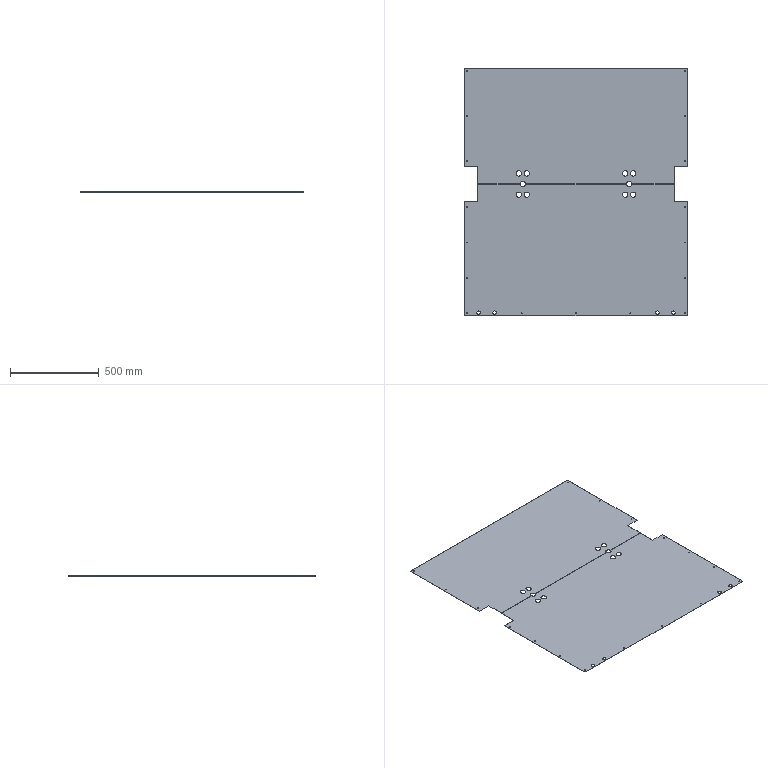Part | SolidWorks | features ICE 4, FlatPattern 2, Cut 1, Fillet 1, MirrorPattern 1, SMBaseFlange 1, SheetMetal 1 | 2 solids | 88 faces | box 1260 x 1400 x 1 mm | volume 1723179 mm3 | cylinder 64 | plane 24 | commonest cylinder face diameters 5 x34 30 x20 20 x8 24 x2